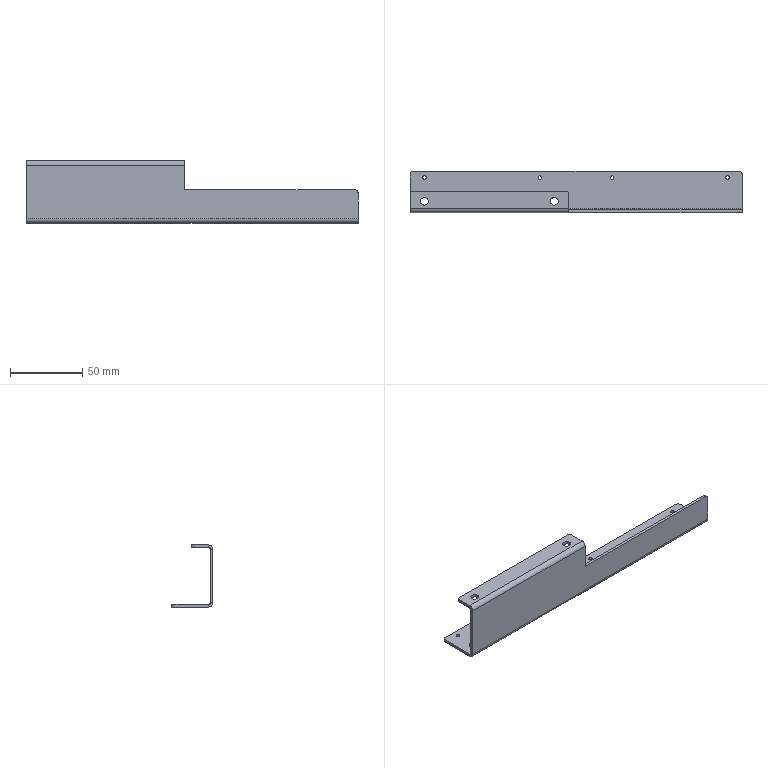Part | SolidWorks | features HoleWzd 2, Cut 1, Fillet 1, FlatPattern 1, SMBaseFlange 1, SheetMetal 1 | 1 solid | 45 faces | box 230 x 29 x 43 mm | volume 29332 mm3 | cylinder 25 | plane 20 | commonest cylinder face diameters 2.5 x8 4 x5 5.5 x4 8 x4 2 x2 6 x2
STEP:
#1=CARTESIAN_POINT('',(11.25,24.5,-19.5));
#2=VERTEX_POINT('',#1);
#3=CARTESIAN_POINT('',(8.75,24.5,-19.5));
#4=VERTEX_POINT('',#3);
#5=CARTESIAN_POINT('',(10.,24.5,-19.5));
#6=DIRECTION('',(0.,0.,-1.));
#7=DIRECTION('',(-1.,0.,0.));
#8=AXIS2_PLACEMENT_3D('',#5,#6,#7);
#9=CIRCLE('',#8,1.25);
#10=EDGE_CURVE('',#2,#4,#9,.T.);
#11=ORIENTED_EDGE('',*,*,#10,.F.);
#12=CARTESIAN_POINT('',(11.25,24.5,-21.5));
#13=VERTEX_POINT('',#12);
#14=CARTESIAN_POINT('',(11.25,24.5,-21.5));
#15=DIRECTION('',(0.,0.,-1.));
#16=VECTOR('',#15,1000.);
#17=LINE('',#14,#16);
#18=EDGE_CURVE('',#2,#13,#17,.T.);
#19=ORIENTED_EDGE('',*,*,#18,.T.);
#20=CARTESIAN_POINT('',(8.75,24.5,-21.5));
#21=VERTEX_POINT('',#20);
#22=CARTESIAN_POINT('',(10.,24.5,-21.5));
#23=DIRECTION('',(0.,0.,-1.));
#24=DIRECTION('',(-1.,0.,0.));
#25=AXIS2_PLACEMENT_3D('',#22,#23,#24);
#26=CIRCLE('',#25,1.25);
#27=EDGE_CURVE('',#13,#21,#26,.T.);
#28=ORIENTED_EDGE('',*,*,#27,.T.);
#29=CARTESIAN_POINT('',(8.75,24.5,-21.5));
#30=DIRECTION('',(0.,0.,-1.));
#31=VECTOR('',#30,1000.);
#32=LINE('',#29,#31);
#33=EDGE_CURVE('',#4,#21,#32,.T.);
#34=ORIENTED_EDGE('',*,*,#33,.F.);
#35=EDGE_LOOP('',(#11,#19,#28,#34));
#36=FACE_OUTER_BOUND('',#35,.T.);
#37=CARTESIAN_POINT('',(10.,24.5,-21.5));
#38=DIRECTION('',(0.,0.,-1.));
#39=DIRECTION('',(-1.,0.,0.));
#40=AXIS2_PLACEMENT_3D('',#37,#38,#39);
#41=CYLINDRICAL_SURFACE('',#40,1.25);
#42=ADVANCED_FACE('',(#36),#41,.F.);
#43=CARTESIAN_POINT('',(91.25,24.5,-19.5));
#44=VERTEX_POINT('',#43);
#45=CARTESIAN_POINT('',(88.75,24.5,-19.5));
#46=VERTEX_POINT('',#45);
#47=CARTESIAN_POINT('',(90.,24.5,-19.5));
#48=DIRECTION('',(0.,0.,-1.));
#49=DIRECTION('',(-1.,0.,0.));
#50=AXIS2_PLACEMENT_3D('',#47,#48,#49);
#51=CIRCLE('',#50,1.25);
#52=EDGE_CURVE('',#44,#46,#51,.T.);
#53=ORIENTED_EDGE('',*,*,#52,.F.);
#54=CARTESIAN_POINT('',(91.25,24.5,-21.5));
#55=VERTEX_POINT('',#54);
#56=CARTESIAN_POINT('',(91.25,24.5,-21.5));
#57=DIRECTION('',(0.,0.,-1.));
#58=VECTOR('',#57,1000.);
#59=LINE('',#56,#58);
#60=EDGE_CURVE('',#44,#55,#59,.T.);
#61=ORIENTED_EDGE('',*,*,#60,.T.);
#62=CARTESIAN_POINT('',(88.75,24.5,-21.5));
#63=VERTEX_POINT('',#62);
#64=CARTESIAN_POINT('',(90.,24.5,-21.5));
#65=DIRECTION('',(0.,0.,-1.));
#66=DIRECTION('',(-1.,0.,0.));
#67=AXIS2_PLACEMENT_3D('',#64,#65,#66);
#68=CIRCLE('',#67,1.25);
#69=EDGE_CURVE('',#55,#63,#68,.T.);
#70=ORIENTED_EDGE('',*,*,#69,.T.);
#71=CARTESIAN_POINT('',(88.75,24.5,-21.5));
#72=DIRECTION('',(0.,0.,-1.));
#73=VECTOR('',#72,1000.);
#74=LINE('',#71,#73);
#75=EDGE_CURVE('',#46,#63,#74,.T.);
#76=ORIENTED_EDGE('',*,*,#75,.F.);
#77=EDGE_LOOP('',(#53,#61,#70,#76));
#78=FACE_OUTER_BOUND('',#77,.T.);
#79=CARTESIAN_POINT('',(90.,24.5,-21.5));
#80=DIRECTION('',(0.,0.,-1.));
#81=DIRECTION('',(-1.,0.,0.));
#82=AXIS2_PLACEMENT_3D('',#79,#80,#81);
#83=CYLINDRICAL_SURFACE('',#82,1.25);
#84=ADVANCED_FACE('',(#78),#83,.F.);
#85=CARTESIAN_POINT('',(141.25,24.5,-19.5));
#86=VERTEX_POINT('',#85);
#87=CARTESIAN_POINT('',(138.75,24.5,-19.5));
#88=VERTEX_POINT('',#87);
#89=CARTESIAN_POINT('',(140.,24.5,-19.5));
#90=DIRECTION('',(0.,0.,-1.));
#91=DIRECTION('',(-1.,0.,0.));
#92=AXIS2_PLACEMENT_3D('',#89,#90,#91);
#93=CIRCLE('',#92,1.25);
#94=EDGE_CURVE('',#86,#88,#93,.T.);
#95=ORIENTED_EDGE('',*,*,#94,.F.);
#96=CARTESIAN_POINT('',(141.25,24.5,-21.5));
#97=VERTEX_POINT('',#96);
#98=CARTESIAN_POINT('',(141.25,24.5,-21.5));
#99=DIRECTION('',(0.,0.,-1.));
#100=VECTOR('',#99,1000.);
#101=LINE('',#98,#100);
#102=EDGE_CURVE('',#86,#97,#101,.T.);
#103=ORIENTED_EDGE('',*,*,#102,.T.);
#104=CARTESIAN_POINT('',(138.75,24.5,-21.5));
#105=VERTEX_POINT('',#104);
#106=CARTESIAN_POINT('',(140.,24.5,-21.5));
#107=DIRECTION('',(0.,0.,-1.));
#108=DIRECTION('',(-1.,0.,0.));
#109=AXIS2_PLACEMENT_3D('',#106,#107,#108);
#110=CIRCLE('',#109,1.25);
#111=EDGE_CURVE('',#97,#105,#110,.T.);
#112=ORIENTED_EDGE('',*,*,#111,.T.);
#113=CARTESIAN_POINT('',(138.75,24.5,-21.5));
#114=DIRECTION('',(0.,0.,-1.));
#115=VECTOR('',#114,1000.);
#116=LINE('',#113,#115);
#117=EDGE_CURVE('',#88,#105,#116,.T.);
#118=ORIENTED_EDGE('',*,*,#117,.F.);
#119=EDGE_LOOP('',(#95,#103,#112,#118));
#120=FACE_OUTER_BOUND('',#119,.T.);
#121=CARTESIAN_POINT('',(140.,24.5,-21.5));
#122=DIRECTION('',(0.,0.,-1.));
#123=DIRECTION('',(-1.,0.,0.));
#124=AXIS2_PLACEMENT_3D('',#121,#122,#123);
#125=CYLINDRICAL_SURFACE('',#124,1.25);
#126=ADVANCED_FACE('',(#120),#125,.F.);
#127=CARTESIAN_POINT('',(221.25,24.5,-19.5));
#128=VERTEX_POINT('',#127);
#129=CARTESIAN_POINT('',(218.75,24.5,-19.5));
#130=VERTEX_POINT('',#129);
#131=CARTESIAN_POINT('',(220.,24.5,-19.5));
#132=DIRECTION('',(0.,0.,-1.));
#133=DIRECTION('',(-1.,0.,0.));
#134=AXIS2_PLACEMENT_3D('',#131,#132,#133);
#135=CIRCLE('',#134,1.25);
#136=EDGE_CURVE('',#128,#130,#135,.T.);
#137=ORIENTED_EDGE('',*,*,#136,.F.);
#138=CARTESIAN_POINT('',(221.25,24.5,-21.5));
#139=VERTEX_POINT('',#138);
#140=CARTESIAN_POINT('',(221.25,24.5,-21.5));
#141=DIRECTION('',(0.,0.,-1.));
#142=VECTOR('',#141,1000.);
#143=LINE('',#140,#142);
#144=EDGE_CURVE('',#128,#139,#143,.T.);
#145=ORIENTED_EDGE('',*,*,#144,.T.);
#146=CARTESIAN_POINT('',(218.75,24.5,-21.5));
#147=VERTEX_POINT('',#146);
#148=CARTESIAN_POINT('',(220.,24.5,-21.5));
#149=DIRECTION('',(0.,0.,-1.));
#150=DIRECTION('',(-1.,0.,0.));
#151=AXIS2_PLACEMENT_3D('',#148,#149,#150);
#152=CIRCLE('',#151,1.25);
#153=EDGE_CURVE('',#139,#147,#152,.T.);
#154=ORIENTED_EDGE('',*,*,#153,.T.);
#155=CARTESIAN_POINT('',(218.75,24.5,-21.5));
#156=DIRECTION('',(0.,0.,-1.));
#157=VECTOR('',#156,1000.);
#158=LINE('',#155,#157);
#159=EDGE_CURVE('',#130,#147,#158,.T.);
#160=ORIENTED_EDGE('',*,*,#159,.F.);
#161=EDGE_LOOP('',(#137,#145,#154,#160));
#162=FACE_OUTER_BOUND('',#161,.T.);
#163=CARTESIAN_POINT('',(220.,24.5,-21.5));
#164=DIRECTION('',(0.,0.,-1.));
#165=DIRECTION('',(-1.,0.,0.));
#166=AXIS2_PLACEMENT_3D('',#163,#164,#165);
#167=CYLINDRICAL_SURFACE('',#166,1.25);
#168=ADVANCED_FACE('',(#162),#167,.F.);
#169=CARTESIAN_POINT('',(12.75,8.,21.5));
#170=VERTEX_POINT('',#169);
#171=CARTESIAN_POINT('',(7.25,8.,21.5));
#172=VERTEX_POINT('',#171);
#173=CARTESIAN_POINT('',(10.,8.,21.5));
#174=DIRECTION('',(0.,0.,-1.));
#175=DIRECTION('',(-1.,0.,0.));
#176=AXIS2_PLACEMENT_3D('',#173,#174,#175);
#177=CIRCLE('',#176,2.75);
#178=EDGE_CURVE('',#170,#172,#177,.T.);
#179=ORIENTED_EDGE('',*,*,#178,.F.);
#180=CARTESIAN_POINT('',(12.75,8.,19.5));
#181=VERTEX_POINT('',#180);
#182=CARTESIAN_POINT('',(12.75,8.,-21.5));
#183=DIRECTION('',(0.,0.,-1.));
#184=VECTOR('',#183,1000.);
#185=LINE('',#182,#184);
#186=EDGE_CURVE('',#170,#181,#185,.T.);
#187=ORIENTED_EDGE('',*,*,#186,.T.);
#188=CARTESIAN_POINT('',(7.25,8.,19.5));
#189=VERTEX_POINT('',#188);
#190=CARTESIAN_POINT('',(10.,8.,19.5));
#191=DIRECTION('',(0.,0.,1.));
#192=DIRECTION('',(1.,0.,0.));
#193=AXIS2_PLACEMENT_3D('',#190,#191,#192);
#194=CIRCLE('',#193,2.75);
#195=EDGE_CURVE('',#189,#181,#194,.T.);
#196=ORIENTED_EDGE('',*,*,#195,.F.);
#197=CARTESIAN_POINT('',(7.25,8.,-21.5));
#198=DIRECTION('',(0.,0.,-1.));
#199=VECTOR('',#198,1000.);
#200=LINE('',#197,#199);
#201=EDGE_CURVE('',#172,#189,#200,.T.);
#202=ORIENTED_EDGE('',*,*,#201,.F.);
#203=EDGE_LOOP('',(#179,#187,#196,#202));
#204=FACE_OUTER_BOUND('',#203,.T.);
#205=CARTESIAN_POINT('',(10.,8.,-21.5));
#206=DIRECTION('',(0.,0.,-1.));
#207=DIRECTION('',(-1.,0.,0.));
#208=AXIS2_PLACEMENT_3D('',#205,#206,#207);
#209=CYLINDRICAL_SURFACE('',#208,2.75);
#210=ADVANCED_FACE('',(#204),#209,.F.);
#211=CARTESIAN_POINT('',(14.,8.,-19.5));
#212=VERTEX_POINT('',#211);
#213=CARTESIAN_POINT('',(6.,8.,-19.5));
#214=VERTEX_POINT('',#213);
#215=CARTESIAN_POINT('',(10.,8.,-19.5));
#216=DIRECTION('',(0.,0.,-1.));
#217=DIRECTION('',(-1.,0.,0.));
#218=AXIS2_PLACEMENT_3D('',#215,#216,#217);
#219=CIRCLE('',#218,4.);
#220=EDGE_CURVE('',#212,#214,#219,.T.);
#221=ORIENTED_EDGE('',*,*,#220,.F.);
#222=CARTESIAN_POINT('',(14.,8.,-21.5));
#223=VERTEX_POINT('',#222);
#224=CARTESIAN_POINT('',(14.,8.,-21.5));
#225=DIRECTION('',(0.,0.,-1.));
#226=VECTOR('',#225,1000.);
#227=LINE('',#224,#226);
#228=EDGE_CURVE('',#212,#223,#227,.T.);
#229=ORIENTED_EDGE('',*,*,#228,.T.);
#230=CARTESIAN_POINT('',(6.,8.,-21.5));
#231=VERTEX_POINT('',#230);
#232=CARTESIAN_POINT('',(10.,8.,-21.5));
#233=DIRECTION('',(0.,0.,-1.));
#234=DIRECTION('',(-1.,0.,0.));
#235=AXIS2_PLACEMENT_3D('',#232,#233,#234);
#236=CIRCLE('',#235,4.);
#237=EDGE_CURVE('',#223,#231,#236,.T.);
#238=ORIENTED_EDGE('',*,*,#237,.T.);
#239=CARTESIAN_POINT('',(6.,8.,-21.5));
#240=DIRECTION('',(0.,0.,-1.));
#241=VECTOR('',#240,1000.);
#242=LINE('',#239,#241);
#243=EDGE_CURVE('',#214,#231,#242,.T.);
#244=ORIENTED_EDGE('',*,*,#243,.F.);
#245=EDGE_LOOP('',(#221,#229,#238,#244));
#246=FACE_OUTER_BOUND('',#245,.T.);
#247=CARTESIAN_POINT('',(10.,8.,-21.5));
#248=DIRECTION('',(0.,0.,-1.));
#249=DIRECTION('',(-1.,0.,0.));
#250=AXIS2_PLACEMENT_3D('',#247,#248,#249);
#251=CYLINDRICAL_SURFACE('',#250,4.);
#252=ADVANCED_FACE('',(#246),#251,.F.);
#253=CARTESIAN_POINT('',(102.75,8.,21.5));
#254=VERTEX_POINT('',#253);
#255=CARTESIAN_POINT('',(97.25,8.,21.5));
#256=VERTEX_POINT('',#255);
#257=CARTESIAN_POINT('',(100.,8.,21.5));
#258=DIRECTION('',(0.,0.,-1.));
#259=DIRECTION('',(-1.,0.,0.));
#260=AXIS2_PLACEMENT_3D('',#257,#258,#259);
#261=CIRCLE('',#260,2.75);
#262=EDGE_CURVE('',#254,#256,#261,.T.);
#263=ORIENTED_EDGE('',*,*,#262,.F.);
#264=CARTESIAN_POINT('',(102.75,8.,19.5));
#265=VERTEX_POINT('',#264);
#266=CARTESIAN_POINT('',(102.75,8.,-21.5));
#267=DIRECTION('',(0.,0.,-1.));
#268=VECTOR('',#267,1000.);
#269=LINE('',#266,#268);
#270=EDGE_CURVE('',#254,#265,#269,.T.);
#271=ORIENTED_EDGE('',*,*,#270,.T.);
#272=CARTESIAN_POINT('',(97.25,8.,19.5));
#273=VERTEX_POINT('',#272);
#274=CARTESIAN_POINT('',(100.,8.,19.5));
#275=DIRECTION('',(0.,0.,1.));
#276=DIRECTION('',(1.,0.,0.));
#277=AXIS2_PLACEMENT_3D('',#274,#275,#276);
#278=CIRCLE('',#277,2.75);
#279=EDGE_CURVE('',#273,#265,#278,.T.);
#280=ORIENTED_EDGE('',*,*,#279,.F.);
#281=CARTESIAN_POINT('',(97.25,8.,-21.5));
#282=DIRECTION('',(0.,0.,-1.));
#283=VECTOR('',#282,1000.);
#284=LINE('',#281,#283);
#285=EDGE_CURVE('',#256,#273,#284,.T.);
#286=ORIENTED_EDGE('',*,*,#285,.F.);
#287=EDGE_LOOP('',(#263,#271,#280,#286));
#288=FACE_OUTER_BOUND('',#287,.T.);
#289=CARTESIAN_POINT('',(100.,8.,-21.5));
#290=DIRECTION('',(0.,0.,-1.));
#291=DIRECTION('',(-1.,0.,0.));
#292=AXIS2_PLACEMENT_3D('',#289,#290,#291);
#293=CYLINDRICAL_SURFACE('',#292,2.75);
#294=ADVANCED_FACE('',(#288),#293,.F.);
#295=CARTESIAN_POINT('',(104.,8.,-19.5));
#296=VERTEX_POINT('',#295);
#297=CARTESIAN_POINT('',(96.,8.,-19.5));
#298=VERTEX_POINT('',#297);
#299=CARTESIAN_POINT('',(100.,8.,-19.5));
#300=DIRECTION('',(0.,0.,-1.));
#301=DIRECTION('',(-1.,0.,0.));
#302=AXIS2_PLACEMENT_3D('',#299,#300,#301);
#303=CIRCLE('',#302,4.);
#304=EDGE_CURVE('',#296,#298,#303,.T.);
#305=ORIENTED_EDGE('',*,*,#304,.F.);
#306=CARTESIAN_POINT('',(104.,8.,-21.5));
#307=VERTEX_POINT('',#306);
#308=CARTESIAN_POINT('',(104.,8.,-21.5));
#309=DIRECTION('',(0.,0.,-1.));
#310=VECTOR('',#309,1000.);
#311=LINE('',#308,#310);
#312=EDGE_CURVE('',#296,#307,#311,.T.);
#313=ORIENTED_EDGE('',*,*,#312,.T.);
#314=CARTESIAN_POINT('',(96.,8.,-21.5));
#315=VERTEX_POINT('',#314);
#316=CARTESIAN_POINT('',(100.,8.,-21.5));
#317=DIRECTION('',(0.,0.,-1.));
#318=DIRECTION('',(-1.,0.,0.));
#319=AXIS2_PLACEMENT_3D('',#316,#317,#318);
#320=CIRCLE('',#319,4.);
#321=EDGE_CURVE('',#307,#315,#320,.T.);
#322=ORIENTED_EDGE('',*,*,#321,.T.);
#323=CARTESIAN_POINT('',(96.,8.,-21.5));
#324=DIRECTION('',(0.,0.,-1.));
#325=VECTOR('',#324,1000.);
#326=LINE('',#323,#325);
#327=EDGE_CURVE('',#298,#315,#326,.T.);
#328=ORIENTED_EDGE('',*,*,#327,.F.);
#329=EDGE_LOOP('',(#305,#313,#322,#328));
#330=FACE_OUTER_BOUND('',#329,.T.);
#331=CARTESIAN_POINT('',(100.,8.,-21.5));
#332=DIRECTION('',(0.,0.,-1.));
#333=DIRECTION('',(-1.,0.,0.));
#334=AXIS2_PLACEMENT_3D('',#331,#332,#333);
#335=CYLINDRICAL_SURFACE('',#334,4.);
#336=ADVANCED_FACE('',(#330),#335,.F.);
#337=CARTESIAN_POINT('',(110.,2.,18.5));
#338=VERTEX_POINT('',#337);
#339=CARTESIAN_POINT('',(110.,2.,1.5));
#340=VERTEX_POINT('',#339);
#341=CARTESIAN_POINT('',(110.,2.,21.5));
#342=DIRECTION('',(0.,0.,-1.));
#343=VECTOR('',#342,1000.);
#344=LINE('',#341,#343);
#345=EDGE_CURVE('',#338,#340,#344,.T.);
#346=ORIENTED_EDGE('',*,*,#345,.F.);
#347=CARTESIAN_POINT('',(110.,0.,18.5));
#348=VERTEX_POINT('',#347);
#349=CARTESIAN_POINT('',(110.,2.,18.5));
#350=DIRECTION('',(0.,-1.,0.));
#351=VECTOR('',#350,1000.);
#352=LINE('',#349,#351);
#353=EDGE_CURVE('',#338,#348,#352,.T.);
#354=ORIENTED_EDGE('',*,*,#353,.T.);
#355=CARTESIAN_POINT('',(110.,0.,1.5));
#356=VERTEX_POINT('',#355);
#357=CARTESIAN_POINT('',(110.,0.,21.5));
#358=DIRECTION('',(0.,0.,-1.));
#359=VECTOR('',#358,1000.);
#360=LINE('',#357,#359);
#361=EDGE_CURVE('',#348,#356,#360,.T.);
#362=ORIENTED_EDGE('',*,*,#361,.T.);
#363=CARTESIAN_POINT('',(110.,29.,1.5));
#364=DIRECTION('',(0.,-1.,0.));
#365=VECTOR('',#364,1000.);
#366=LINE('',#363,#365);
#367=EDGE_CURVE('',#340,#356,#366,.T.);
#368=ORIENTED_EDGE('',*,*,#367,.F.);
#369=EDGE_LOOP('',(#346,#354,#362,#368));
#370=FACE_OUTER_BOUND('',#369,.T.);
#371=CARTESIAN_POINT('',(110.,29.,21.5));
#372=DIRECTION('',(-1.,0.,0.));
#373=DIRECTION('',(0.,0.,1.));
#374=AXIS2_PLACEMENT_3D('',#371,#372,#373);
#375=PLANE('',#374);
#376=ADVANCED_FACE('',(#370),#375,.F.);
#377=CARTESIAN_POINT('',(110.,13.,19.5));
#378=VERTEX_POINT('',#377);
#379=CARTESIAN_POINT('',(110.,3.,19.5));
#380=VERTEX_POINT('',#379);
#381=CARTESIAN_POINT('',(110.,0.,19.5));
#382=DIRECTION('',(0.,-1.,0.));
#383=VECTOR('',#382,1000.);
#384=LINE('',#381,#383);
#385=EDGE_CURVE('',#378,#380,#384,.T.);
#386=ORIENTED_EDGE('',*,*,#385,.F.);
#387=CARTESIAN_POINT('',(110.,13.,21.5));
#388=VERTEX_POINT('',#387);
#389=CARTESIAN_POINT('',(110.,13.,21.5));
#390=DIRECTION('',(0.,0.,1.));
#391=VECTOR('',#390,1000.);
#392=LINE('',#389,#391);
#393=EDGE_CURVE('',#378,#388,#392,.T.);
#394=ORIENTED_EDGE('',*,*,#393,.T.);
#395=CARTESIAN_POINT('',(110.,3.,21.5));
#396=VERTEX_POINT('',#395);
#397=CARTESIAN_POINT('',(110.,29.,21.5));
#398=DIRECTION('',(0.,-1.,0.));
#399=VECTOR('',#398,1000.);
#400=LINE('',#397,#399);
#401=EDGE_CURVE('',#388,#396,#400,.T.);
#402=ORIENTED_EDGE('',*,*,#401,.T.);
#403=CARTESIAN_POINT('',(110.,3.,21.5));
#404=DIRECTION('',(0.,0.,-1.));
#405=VECTOR('',#404,1000.);
#406=LINE('',#403,#405);
#407=EDGE_CURVE('',#396,#380,#406,.T.);
#408=ORIENTED_EDGE('',*,*,#407,.T.);
#409=EDGE_LOOP('',(#386,#394,#402,#408));
#410=FACE_OUTER_BOUND('',#409,.T.);
#411=CARTESIAN_POINT('',(110.,29.,21.5));
#412=DIRECTION('',(-1.,0.,0.));
#413=DIRECTION('',(0.,0.,1.));
#414=AXIS2_PLACEMENT_3D('',#411,#412,#413);
#415=PLANE('',#414);
#416=ADVANCED_FACE('',(#410),#415,.F.);
#417=CARTESIAN_POINT('',(230.,0.,-18.5));
#418=VERTEX_POINT('',#417);
#419=CARTESIAN_POINT('',(230.,2.,-18.5));
#420=VERTEX_POINT('',#419);
#421=CARTESIAN_POINT('',(230.,0.,-18.5));
#422=DIRECTION('',(0.,1.,0.));
#423=VECTOR('',#422,1000.);
#424=LINE('',#421,#423);
#425=EDGE_CURVE('',#418,#420,#424,.T.);
#426=ORIENTED_EDGE('',*,*,#425,.F.);
#427=CARTESIAN_POINT('',(230.,3.,-21.5));
#428=VERTEX_POINT('',#427);
#429=CARTESIAN_POINT('',(230.,3.,-18.5));
#430=DIRECTION('',(-1.,0.,0.));
#431=DIRECTION('',(0.,0.,-1.));
#432=AXIS2_PLACEMENT_3D('',#429,#430,#431);
#433=CIRCLE('',#432,3.);
#434=EDGE_CURVE('',#428,#418,#433,.T.);
#435=ORIENTED_EDGE('',*,*,#434,.F.);
#436=CARTESIAN_POINT('',(230.,3.,-19.5));
#437=VERTEX_POINT('',#436);
#438=CARTESIAN_POINT('',(230.,3.,-19.5));
#439=DIRECTION('',(0.,0.,-1.));
#440=VECTOR('',#439,1000.);
#441=LINE('',#438,#440);
#442=EDGE_CURVE('',#437,#428,#441,.T.);
#443=ORIENTED_EDGE('',*,*,#442,.F.);
#444=CARTESIAN_POINT('',(230.,3.,-18.5));
#445=DIRECTION('',(-1.,0.,0.));
#446=DIRECTION('',(0.,0.,-1.));
#447=AXIS2_PLACEMENT_3D('',#444,#445,#446);
#448=CIRCLE('',#447,1.);
#449=EDGE_CURVE('',#437,#420,#448,.T.);
#450=ORIENTED_EDGE('',*,*,#449,.T.);
#451=EDGE_LOOP('',(#426,#435,#443,#450));
#452=FACE_OUTER_BOUND('',#451,.T.);
#453=CARTESIAN_POINT('',(230.,0.,-18.5));
#454=DIRECTION('',(1.,0.,0.));
#455=DIRECTION('',(0.,0.,-1.));
#456=AXIS2_PLACEMENT_3D('',#453,#454,#455);
#457=PLANE('',#456);
#458=ADVANCED_FACE('',(#452),#457,.T.);
#459=CARTESIAN_POINT('',(230.,2.,-0.5));
#460=VERTEX_POINT('',#459);
#461=CARTESIAN_POINT('',(230.,2.,21.5));
#462=DIRECTION('',(0.,0.,1.));
#463=VECTOR('',#462,1000.);
#464=LINE('',#461,#463);
#465=EDGE_CURVE('',#420,#460,#464,.T.);
#466=ORIENTED_EDGE('',*,*,#465,.T.);
#467=CARTESIAN_POINT('',(230.,0.,-0.5));
#468=VERTEX_POINT('',#467);
#469=CARTESIAN_POINT('',(230.,0.,-0.5));
#470=DIRECTION('',(0.,-1.,0.));
#471=VECTOR('',#470,1000.);
#472=LINE('',#469,#471);
#473=EDGE_CURVE('',#460,#468,#472,.T.);
#474=ORIENTED_EDGE('',*,*,#473,.T.);
#475=CARTESIAN_POINT('',(230.,0.,21.5));
#476=DIRECTION('',(0.,0.,1.));
#477=VECTOR('',#476,1000.);
#478=LINE('',#475,#477);
#479=EDGE_CURVE('',#418,#468,#478,.T.);
#480=ORIENTED_EDGE('',*,*,#479,.F.);
#481=ORIENTED_EDGE('',*,*,#425,.T.);
#482=EDGE_LOOP('',(#466,#474,#480,#481));
#483=FACE_OUTER_BOUND('',#482,.T.);
#484=CARTESIAN_POINT('',(230.,3.,-19.5));
#485=DIRECTION('',(1.,0.,0.));
#486=DIRECTION('',(0.,0.,-1.));
#487=AXIS2_PLACEMENT_3D('',#484,#485,#486);
#488=PLANE('',#487);
#489=ADVANCED_FACE('',(#483),#488,.T.);
#490=CARTESIAN_POINT('',(0.,3.,-21.5));
#491=VERTEX_POINT('',#490);
#492=CARTESIAN_POINT('',(0.,3.,-19.5));
#493=VERTEX_POINT('',#492);
#494=CARTESIAN_POINT('',(0.,3.,-21.5));
#495=DIRECTION('',(0.,0.,1.));
#496=VECTOR('',#495,1000.);
#497=LINE('',#494,#496);
#498=EDGE_CURVE('',#491,#493,#497,.T.);
#499=ORIENTED_EDGE('',*,*,#498,.F.);
#500=CARTESIAN_POINT('',(0.,0.,-18.5));
#501=VERTEX_POINT('',#500);
#502=CARTESIAN_POINT('',(0.,3.,-18.5));
#503=DIRECTION('',(-1.,0.,0.));
#504=DIRECTION('',(0.,0.,-1.));
#505=AXIS2_PLACEMENT_3D('',#502,#503,#504);
#506=CIRCLE('',#505,3.);
#507=EDGE_CURVE('',#491,#501,#506,.T.);
#508=ORIENTED_EDGE('',*,*,#507,.T.);
#509=CARTESIAN_POINT('',(0.,2.,-18.5));
#510=VERTEX_POINT('',#509);
#511=CARTESIAN_POINT('',(0.,2.,-18.5));
#512=DIRECTION('',(0.,-1.,0.));
#513=VECTOR('',#512,1000.);
#514=LINE('',#511,#513);
#515=EDGE_CURVE('',#510,#501,#514,.T.);
#516=ORIENTED_EDGE('',*,*,#515,.F.);
#517=CARTESIAN_POINT('',(0.,3.,-18.5));
#518=DIRECTION('',(-1.,0.,0.));
#519=DIRECTION('',(0.,0.,-1.));
#520=AXIS2_PLACEMENT_3D('',#517,#518,#519);
#521=CIRCLE('',#520,1.);
#522=EDGE_CURVE('',#493,#510,#521,.T.);
#523=ORIENTED_EDGE('',*,*,#522,.F.);
#524=EDGE_LOOP('',(#499,#508,#516,#523));
#525=FACE_OUTER_BOUND('',#524,.T.);
#526=CARTESIAN_POINT('',(0.,3.,-21.5));
#527=DIRECTION('',(-1.,0.,0.));
#528=DIRECTION('',(0.,0.,1.));
#529=AXIS2_PLACEMENT_3D('',#526,#527,#528);
#530=PLANE('',#529);
#531=ADVANCED_FACE('',(#525),#530,.T.);
#532=CARTESIAN_POINT('',(0.,27.,-19.5));
#533=VERTEX_POINT('',#532);
#534=CARTESIAN_POINT('',(0.,0.,-19.5));
#535=DIRECTION('',(0.,-1.,0.));
#536=VECTOR('',#535,1000.);
#537=LINE('',#534,#536);
#538=EDGE_CURVE('',#533,#493,#537,.T.);
#539=ORIENTED_EDGE('',*,*,#538,.F.);
#540=CARTESIAN_POINT('',(0.,27.,-21.5));
#541=VERTEX_POINT('',#540);
#542=CARTESIAN_POINT('',(0.,27.,-18.5));
#543=DIRECTION('',(0.,0.,-1.));
#544=VECTOR('',#543,1000.);
#545=LINE('',#542,#544);
#546=EDGE_CURVE('',#533,#541,#545,.T.);
#547=ORIENTED_EDGE('',*,*,#546,.T.);
#548=CARTESIAN_POINT('',(0.,0.,-21.5));
#549=DIRECTION('',(0.,-1.,0.));
#550=VECTOR('',#549,1000.);
#551=LINE('',#548,#550);
#552=EDGE_CURVE('',#541,#491,#551,.T.);
#553=ORIENTED_EDGE('',*,*,#552,.T.);
#554=ORIENTED_EDGE('',*,*,#498,.T.);
#555=EDGE_LOOP('',(#539,#547,#553,#554));
#556=FACE_OUTER_BOUND('',#555,.T.);
#557=CARTESIAN_POINT('',(0.,2.,-18.5));
#558=DIRECTION('',(-1.,0.,0.));
#559=DIRECTION('',(0.,0.,1.));
#560=AXIS2_PLACEMENT_3D('',#557,#558,#559);
#561=PLANE('',#560);
#562=ADVANCED_FACE('',(#556),#561,.T.);
#563=CARTESIAN_POINT('',(0.,0.,18.5));
#564=VERTEX_POINT('',#563);
#565=CARTESIAN_POINT('',(0.,2.,18.5));
#566=VERTEX_POINT('',#565);
#567=CARTESIAN_POINT('',(0.,0.,18.5));
#568=DIRECTION('',(0.,1.,0.));
#569=VECTOR('',#568,1000.);
#570=LINE('',#567,#569);
#571=EDGE_CURVE('',#564,#566,#570,.T.);
#572=ORIENTED_EDGE('',*,*,#571,.F.);
#573=CARTESIAN_POINT('',(0.,3.,21.5));
#574=VERTEX_POINT('',#573);
#575=CARTESIAN_POINT('',(0.,3.,18.5));
#576=DIRECTION('',(-1.,0.,0.));
#577=DIRECTION('',(0.,0.,-1.));
#578=AXIS2_PLACEMENT_3D('',#575,#576,#577);
#579=CIRCLE('',#578,3.);
#580=EDGE_CURVE('',#564,#574,#579,.T.);
#581=ORIENTED_EDGE('',*,*,#580,.T.);
#582=CARTESIAN_POINT('',(0.,3.,19.5));
#583=VERTEX_POINT('',#582);
#584=CARTESIAN_POINT('',(0.,3.,19.5));
#585=DIRECTION('',(0.,0.,1.));
#586=VECTOR('',#585,1000.);
#587=LINE('',#584,#586);
#588=EDGE_CURVE('',#583,#574,#587,.T.);
#589=ORIENTED_EDGE('',*,*,#588,.F.);
#590=CARTESIAN_POINT('',(0.,3.,18.5));
#591=DIRECTION('',(-1.,0.,0.));
#592=DIRECTION('',(0.,0.,-1.));
#593=AXIS2_PLACEMENT_3D('',#590,#591,#592);
#594=CIRCLE('',#593,1.);
#595=EDGE_CURVE('',#566,#583,#594,.T.);
#596=ORIENTED_EDGE('',*,*,#595,.F.);
#597=EDGE_LOOP('',(#572,#581,#589,#596));
#598=FACE_OUTER_BOUND('',#597,.T.);
#599=CARTESIAN_POINT('',(0.,0.,18.5));
#600=DIRECTION('',(-1.,0.,0.));
#601=DIRECTION('',(0.,0.,1.));
#602=AXIS2_PLACEMENT_3D('',#599,#600,#601);
#603=PLANE('',#602);
#604=ADVANCED_FACE('',(#598),#603,.T.);
#605=CARTESIAN_POINT('',(0.,0.,21.5));
#606=DIRECTION('',(0.,0.,1.));
#607=VECTOR('',#606,1000.);
#608=LINE('',#605,#607);
#609=EDGE_CURVE('',#501,#564,#608,.T.);
#610=ORIENTED_EDGE('',*,*,#609,.T.);
#611=ORIENTED_EDGE('',*,*,#571,.T.);
#612=CARTESIAN_POINT('',(0.,2.,21.5));
#613=DIRECTION('',(0.,0.,1.));
#614=VECTOR('',#613,1000.);
#615=LINE('',#612,#614);
#616=EDGE_CURVE('',#510,#566,#615,.T.);
#617=ORIENTED_EDGE('',*,*,#616,.F.);
#618=ORIENTED_EDGE('',*,*,#515,.T.);
#619=EDGE_LOOP('',(#610,#611,#617,#618));
#620=FACE_OUTER_BOUND('',#619,.T.);
#621=CARTESIAN_POINT('',(0.,3.,19.5));
#622=DIRECTION('',(-1.,0.,0.));
#623=DIRECTION('',(0.,0.,1.));
#624=AXIS2_PLACEMENT_3D('',#621,#622,#623);
#625=PLANE('',#624);
#626=ADVANCED_FACE('',(#620),#625,.T.);
#627=ORIENTED_EDGE('',*,*,#195,.T.);
#628=CARTESIAN_POINT('',(10.,8.,19.5));
#629=DIRECTION('',(0.,0.,1.));
#630=DIRECTION('',(1.,0.,0.));
#631=AXIS2_PLACEMENT_3D('',#628,#629,#630);
#632=CIRCLE('',#631,2.75);
#633=EDGE_CURVE('',#181,#189,#632,.T.);
#634=ORIENTED_EDGE('',*,*,#633,.T.);
#635=EDGE_LOOP('',(#627,#634));
#636=FACE_BOUND('',#635,.T.);
#637=ORIENTED_EDGE('',*,*,#279,.T.);
#638=CARTESIAN_POINT('',(100.,8.,19.5));
#639=DIRECTION('',(0.,0.,1.));
#640=DIRECTION('',(1.,0.,0.));
#641=AXIS2_PLACEMENT_3D('',#638,#639,#640);
#642=CIRCLE('',#641,2.75);
#643=EDGE_CURVE('',#265,#273,#642,.T.);
#644=ORIENTED_EDGE('',*,*,#643,.T.);
#645=EDGE_LOOP('',(#637,#644));
#646=FACE_BOUND('',#645,.T.);
#647=CARTESIAN_POINT('',(108.,15.,19.5));
#648=VERTEX_POINT('',#647);
#649=CARTESIAN_POINT('',(2.,15.,19.5));
#650=VERTEX_POINT('',#649);
#651=CARTESIAN_POINT('',(230.,15.,19.5));
#652=DIRECTION('',(-1.,0.,0.));
#653=VECTOR('',#652,1000.);
#654=LINE('',#651,#653);
#655=EDGE_CURVE('',#648,#650,#654,.T.);
#656=ORIENTED_EDGE('',*,*,#655,.F.);
#657=CARTESIAN_POINT('',(108.,13.,19.5));
#658=DIRECTION('',(0.,0.,-1.));
#659=DIRECTION('',(1.,0.,0.));
#660=AXIS2_PLACEMENT_3D('',#657,#658,#659);
#661=CIRCLE('',#660,2.);
#662=EDGE_CURVE('',#648,#378,#661,.T.);
#663=ORIENTED_EDGE('',*,*,#662,.T.);
#664=ORIENTED_EDGE('',*,*,#385,.T.);
#665=CARTESIAN_POINT('',(230.,3.,19.5));
#666=DIRECTION('',(-1.,0.,0.));
#667=VECTOR('',#666,1000.);
#668=LINE('',#665,#667);
#669=EDGE_CURVE('',#380,#583,#668,.T.);
#670=ORIENTED_EDGE('',*,*,#669,.T.);
#671=CARTESIAN_POINT('',(0.,13.,19.5));
#672=VERTEX_POINT('',#671);
#673=CARTESIAN_POINT('',(0.,0.,19.5));
#674=DIRECTION('',(0.,1.,0.));
#675=VECTOR('',#674,1000.);
#676=LINE('',#673,#675);
#677=EDGE_CURVE('',#583,#672,#676,.T.);
#678=ORIENTED_EDGE('',*,*,#677,.T.);
#679=CARTESIAN_POINT('',(2.,13.,19.5));
#680=DIRECTION('',(0.,0.,-1.));
#681=DIRECTION('',(1.,0.,0.));
#682=AXIS2_PLACEMENT_3D('',#679,#680,#681);
#683=CIRCLE('',#682,2.);
#684=EDGE_CURVE('',#672,#650,#683,.T.);
#685=ORIENTED_EDGE('',*,*,#684,.T.);
#686=EDGE_LOOP('',(#656,#663,#664,#670,#678,#685));
#687=FACE_OUTER_BOUND('',#686,.T.);
#688=CARTESIAN_POINT('',(230.,0.,19.5));
#689=DIRECTION('',(0.,0.,1.));
#690=DIRECTION('',(1.,0.,0.));
#691=AXIS2_PLACEMENT_3D('',#688,#689,#690);
#692=PLANE('',#691);
#693=ADVANCED_FACE('',(#636,#646,#687),#692,.F.);
#694=CARTESIAN_POINT('',(108.,15.,21.5));
#695=VERTEX_POINT('',#694);
#696=CARTESIAN_POINT('',(2.,15.,21.5));
#697=VERTEX_POINT('',#696);
#698=CARTESIAN_POINT('',(230.,15.,21.5));
#699=DIRECTION('',(-1.,0.,0.));
#700=VECTOR('',#699,1000.);
#701=LINE('',#698,#700);
#702=EDGE_CURVE('',#695,#697,#701,.T.);
#703=ORIENTED_EDGE('',*,*,#702,.F.);
#704=CARTESIAN_POINT('',(108.,15.,19.5));
#705=DIRECTION('',(0.,0.,-1.));
#706=VECTOR('',#705,1000.);
#707=LINE('',#704,#706);
#708=EDGE_CURVE('',#695,#648,#707,.T.);
#709=ORIENTED_EDGE('',*,*,#708,.T.);
#710=ORIENTED_EDGE('',*,*,#655,.T.);
#711=CARTESIAN_POINT('',(2.,15.,21.5));
#712=DIRECTION('',(0.,0.,1.));
#713=VECTOR('',#712,1000.);
#714=LINE('',#711,#713);
#715=EDGE_CURVE('',#650,#697,#714,.T.);
#716=ORIENTED_EDGE('',*,*,#715,.T.);
#717=EDGE_LOOP('',(#703,#709,#710,#716));
#718=FACE_OUTER_BOUND('',#717,.T.);
#719=CARTESIAN_POINT('',(230.,15.,21.5));
#720=DIRECTION('',(0.,1.,0.));
#721=DIRECTION('',(0.,0.,1.));
#722=AXIS2_PLACEMENT_3D('',#719,#720,#721);
#723=PLANE('',#722);
#724=ADVANCED_FACE('',(#718),#723,.T.);
#725=CARTESIAN_POINT('',(10.,8.,21.5));
#726=DIRECTION('',(0.,0.,-1.));
#727=DIRECTION('',(-1.,0.,0.));
#728=AXIS2_PLACEMENT_3D('',#725,#726,#727);
#729=CIRCLE('',#728,2.75);
#730=EDGE_CURVE('',#172,#170,#729,.T.);
#731=ORIENTED_EDGE('',*,*,#730,.T.);
#732=ORIENTED_EDGE('',*,*,#178,.T.);
#733=EDGE_LOOP('',(#731,#732));
#734=FACE_BOUND('',#733,.T.);
#735=CARTESIAN_POINT('',(100.,8.,21.5));
#736=DIRECTION('',(0.,0.,-1.));
#737=DIRECTION('',(-1.,0.,0.));
#738=AXIS2_PLACEMENT_3D('',#735,#736,#737);
#739=CIRCLE('',#738,2.75);
#740=EDGE_CURVE('',#256,#254,#739,.T.);
#741=ORIENTED_EDGE('',*,*,#740,.T.);
#742=ORIENTED_EDGE('',*,*,#262,.T.);
#743=EDGE_LOOP('',(#741,#742));
#744=FACE_BOUND('',#743,.T.);
#745=ORIENTED_EDGE('',*,*,#401,.F.);
#746=CARTESIAN_POINT('',(108.,13.,21.5));
#747=DIRECTION('',(0.,0.,1.));
#748=DIRECTION('',(1.,0.,0.));
#749=AXIS2_PLACEMENT_3D('',#746,#747,#748);
#750=CIRCLE('',#749,2.);
#751=EDGE_CURVE('',#388,#695,#750,.T.);
#752=ORIENTED_EDGE('',*,*,#751,.T.);
#753=ORIENTED_EDGE('',*,*,#702,.T.);
#754=CARTESIAN_POINT('',(0.,13.,21.5));
#755=VERTEX_POINT('',#754);
#756=CARTESIAN_POINT('',(2.,13.,21.5));
#757=DIRECTION('',(0.,0.,1.));
#758=DIRECTION('',(1.,0.,0.));
#759=AXIS2_PLACEMENT_3D('',#756,#757,#758);
#760=CIRCLE('',#759,2.);
#761=EDGE_CURVE('',#697,#755,#760,.T.);
#762=ORIENTED_EDGE('',*,*,#761,.T.);
#763=CARTESIAN_POINT('',(0.,0.,21.5));
#764=DIRECTION('',(0.,1.,0.));
#765=VECTOR('',#764,1000.);
#766=LINE('',#763,#765);
#767=EDGE_CURVE('',#574,#755,#766,.T.);
#768=ORIENTED_EDGE('',*,*,#767,.F.);
#769=CARTESIAN_POINT('',(230.,3.,21.5));
#770=DIRECTION('',(-1.,0.,0.));
#771=VECTOR('',#770,1000.);
#772=LINE('',#769,#771);
#773=EDGE_CURVE('',#396,#574,#772,.T.);
#774=ORIENTED_EDGE('',*,*,#773,.F.);
#775=EDGE_LOOP('',(#745,#752,#753,#762,#768,#774));
#776=FACE_OUTER_BOUND('',#775,.T.);
#777=CARTESIAN_POINT('',(230.,0.,21.5));
#778=DIRECTION('',(0.,0.,1.));
#779=DIRECTION('',(1.,0.,0.));
#780=AXIS2_PLACEMENT_3D('',#777,#778,#779);
#781=PLANE('',#780);
#782=ADVANCED_FACE('',(#734,#744,#776),#781,.T.);
#783=CARTESIAN_POINT('',(110.,3.,18.5));
#784=DIRECTION('',(1.,0.,0.));
#785=DIRECTION('',(0.,0.,1.));
#786=AXIS2_PLACEMENT_3D('',#783,#784,#785);
#787=CIRCLE('',#786,3.);
#788=EDGE_CURVE('',#396,#348,#787,.T.);
#789=ORIENTED_EDGE('',*,*,#788,.F.);
#790=ORIENTED_EDGE('',*,*,#773,.T.);
#791=ORIENTED_EDGE('',*,*,#580,.F.);
#792=CARTESIAN_POINT('',(230.,0.,18.5));
#793=DIRECTION('',(-1.,0.,0.));
#794=VECTOR('',#793,1000.);
#795=LINE('',#792,#794);
#796=EDGE_CURVE('',#348,#564,#795,.T.);
#797=ORIENTED_EDGE('',*,*,#796,.F.);
#798=EDGE_LOOP('',(#789,#790,#791,#797));
#799=FACE_OUTER_BOUND('',#798,.T.);
#800=CARTESIAN_POINT('',(230.,3.,18.5));
#801=DIRECTION('',(-1.,0.,0.));
#802=DIRECTION('',(0.,0.,1.));
#803=AXIS2_PLACEMENT_3D('',#800,#801,#802);
#804=CYLINDRICAL_SURFACE('',#803,3.);
#805=ADVANCED_FACE('',(#799),#804,.T.);
#806=ORIENTED_EDGE('',*,*,#479,.T.);
#807=CARTESIAN_POINT('',(228.,0.,1.5));
#808=VERTEX_POINT('',#807);
#809=CARTESIAN_POINT('',(228.,0.,-0.5));
#810=DIRECTION('',(0.,-1.,0.));
#811=DIRECTION('',(0.,0.,-1.));
#812=AXIS2_PLACEMENT_3D('',#809,#810,#811);
#813=CIRCLE('',#812,2.);
#814=EDGE_CURVE('',#468,#808,#813,.T.);
#815=ORIENTED_EDGE('',*,*,#814,.T.);
#816=CARTESIAN_POINT('',(230.,0.,1.5));
#817=DIRECTION('',(1.,0.,0.));
#818=VECTOR('',#817,1000.);
#819=LINE('',#816,#818);
#820=EDGE_CURVE('',#356,#808,#819,.T.);
#821=ORIENTED_EDGE('',*,*,#820,.F.);
#822=ORIENTED_EDGE('',*,*,#361,.F.);
#823=ORIENTED_EDGE('',*,*,#796,.T.);
#824=ORIENTED_EDGE('',*,*,#609,.F.);
#825=CARTESIAN_POINT('',(230.,0.,-18.5));
#826=DIRECTION('',(-1.,0.,0.));
#827=VECTOR('',#826,1000.);
#828=LINE('',#825,#827);
#829=EDGE_CURVE('',#418,#501,#828,.T.);
#830=ORIENTED_EDGE('',*,*,#829,.F.);
#831=EDGE_LOOP('',(#806,#815,#821,#822,#823,#824,#830));
#832=FACE_OUTER_BOUND('',#831,.T.);
#833=CARTESIAN_POINT('',(230.,0.,21.5));
#834=DIRECTION('',(0.,-1.,0.));
#835=DIRECTION('',(0.,0.,-1.));
#836=AXIS2_PLACEMENT_3D('',#833,#834,#835);
#837=PLANE('',#836);
#838=ADVANCED_FACE('',(#832),#837,.T.);
#839=ORIENTED_EDGE('',*,*,#507,.F.);
#840=CARTESIAN_POINT('',(230.,3.,-21.5));
#841=DIRECTION('',(-1.,0.,0.));
#842=VECTOR('',#841,1000.);
#843=LINE('',#840,#842);
#844=EDGE_CURVE('',#428,#491,#843,.T.);
#845=ORIENTED_EDGE('',*,*,#844,.F.);
#846=ORIENTED_EDGE('',*,*,#434,.T.);
#847=ORIENTED_EDGE('',*,*,#829,.T.);
#848=EDGE_LOOP('',(#839,#845,#846,#847));
#849=FACE_OUTER_BOUND('',#848,.T.);
#850=CARTESIAN_POINT('',(230.,3.,-18.5));
#851=DIRECTION('',(-1.,0.,0.));
#852=DIRECTION('',(0.,0.,1.));
#853=AXIS2_PLACEMENT_3D('',#850,#851,#852);
#854=CYLINDRICAL_SURFACE('',#853,3.);
#855=ADVANCED_FACE('',(#849),#854,.T.);
#856=CARTESIAN_POINT('',(10.,24.5,-21.5));
#857=DIRECTION('',(0.,0.,-1.));
#858=DIRECTION('',(-1.,0.,0.));
#859=AXIS2_PLACEMENT_3D('',#856,#857,#858);
#860=CIRCLE('',#859,1.25);
#861=EDGE_CURVE('',#21,#13,#860,.T.);
#862=ORIENTED_EDGE('',*,*,#861,.F.);
#863=ORIENTED_EDGE('',*,*,#27,.F.);
#864=EDGE_LOOP('',(#862,#863));
#865=FACE_BOUND('',#864,.T.);
#866=CARTESIAN_POINT('',(90.,24.5,-21.5));
#867=DIRECTION('',(0.,0.,-1.));
#868=DIRECTION('',(-1.,0.,0.));
#869=AXIS2_PLACEMENT_3D('',#866,#867,#868);
#870=CIRCLE('',#869,1.25);
#871=EDGE_CURVE('',#63,#55,#870,.T.);
#872=ORIENTED_EDGE('',*,*,#871,.F.);
#873=ORIENTED_EDGE('',*,*,#69,.F.);
#874=EDGE_LOOP('',(#872,#873));
#875=FACE_BOUND('',#874,.T.);
#876=CARTESIAN_POINT('',(140.,24.5,-21.5));
#877=DIRECTION('',(0.,0.,-1.));
#878=DIRECTION('',(-1.,0.,0.));
#879=AXIS2_PLACEMENT_3D('',#876,#877,#878);
#880=CIRCLE('',#879,1.25);
#881=EDGE_CURVE('',#105,#97,#880,.T.);
#882=ORIENTED_EDGE('',*,*,#881,.F.);
#883=ORIENTED_EDGE('',*,*,#111,.F.);
#884=EDGE_LOOP('',(#882,#883));
#885=FACE_BOUND('',#884,.T.);
#886=CARTESIAN_POINT('',(220.,24.5,-21.5));
#887=DIRECTION('',(0.,0.,-1.));
#888=DIRECTION('',(-1.,0.,0.));
#889=AXIS2_PLACEMENT_3D('',#886,#887,#888);
#890=CIRCLE('',#889,1.25);
#891=EDGE_CURVE('',#147,#139,#890,.T.);
#892=ORIENTED_EDGE('',*,*,#891,.F.);
#893=ORIENTED_EDGE('',*,*,#153,.F.);
#894=EDGE_LOOP('',(#892,#893));
#895=FACE_BOUND('',#894,.T.);
#896=CARTESIAN_POINT('',(10.,8.,-21.5));
#897=DIRECTION('',(0.,0.,-1.));
#898=DIRECTION('',(-1.,0.,0.));
#899=AXIS2_PLACEMENT_3D('',#896,#897,#898);
#900=CIRCLE('',#899,4.);
#901=EDGE_CURVE('',#231,#223,#900,.T.);
#902=ORIENTED_EDGE('',*,*,#901,.F.);
#903=ORIENTED_EDGE('',*,*,#237,.F.);
#904=EDGE_LOOP('',(#902,#903));
#905=FACE_BOUND('',#904,.T.);
#906=CARTESIAN_POINT('',(100.,8.,-21.5));
#907=DIRECTION('',(0.,0.,-1.));
#908=DIRECTION('',(-1.,0.,0.));
#909=AXIS2_PLACEMENT_3D('',#906,#907,#908);
#910=CIRCLE('',#909,4.);
#911=EDGE_CURVE('',#315,#307,#910,.T.);
#912=ORIENTED_EDGE('',*,*,#911,.F.);
#913=ORIENTED_EDGE('',*,*,#321,.F.);
#914=EDGE_LOOP('',(#912,#913));
#915=FACE_BOUND('',#914,.T.);
#916=ORIENTED_EDGE('',*,*,#552,.F.);
#917=CARTESIAN_POINT('',(2.,29.,-21.5));
#918=VERTEX_POINT('',#917);
#919=CARTESIAN_POINT('',(2.,27.,-21.5));
#920=DIRECTION('',(0.,0.,-1.));
#921=DIRECTION('',(-1.,0.,0.));
#922=AXIS2_PLACEMENT_3D('',#919,#920,#921);
#923=CIRCLE('',#922,2.);
#924=EDGE_CURVE('',#541,#918,#923,.T.);
#925=ORIENTED_EDGE('',*,*,#924,.T.);
#926=CARTESIAN_POINT('',(228.,29.,-21.5));
#927=VERTEX_POINT('',#926);
#928=CARTESIAN_POINT('',(230.,29.,-21.5));
#929=DIRECTION('',(-1.,0.,0.));
#930=VECTOR('',#929,1000.);
#931=LINE('',#928,#930);
#932=EDGE_CURVE('',#927,#918,#931,.T.);
#933=ORIENTED_EDGE('',*,*,#932,.F.);
#934=CARTESIAN_POINT('',(230.,27.,-21.5));
#935=VERTEX_POINT('',#934);
#936=CARTESIAN_POINT('',(228.,27.,-21.5));
#937=DIRECTION('',(0.,0.,-1.));
#938=DIRECTION('',(-1.,0.,0.));
#939=AXIS2_PLACEMENT_3D('',#936,#937,#938);
#940=CIRCLE('',#939,2.);
#941=EDGE_CURVE('',#927,#935,#940,.T.);
#942=ORIENTED_EDGE('',*,*,#941,.T.);
#943=CARTESIAN_POINT('',(230.,0.,-21.5));
#944=DIRECTION('',(0.,-1.,0.));
#945=VECTOR('',#944,1000.);
#946=LINE('',#943,#945);
#947=EDGE_CURVE('',#935,#428,#946,.T.);
#948=ORIENTED_EDGE('',*,*,#947,.T.);
#949=ORIENTED_EDGE('',*,*,#844,.T.);
#950=EDGE_LOOP('',(#916,#925,#933,#942,#948,#949));
#951=FACE_OUTER_BOUND('',#950,.T.);
#952=CARTESIAN_POINT('',(230.,0.,-21.5));
#953=DIRECTION('',(0.,0.,-1.));
#954=DIRECTION('',(-1.,0.,0.));
#955=AXIS2_PLACEMENT_3D('',#952,#953,#954);
#956=PLANE('',#955);
#957=ADVANCED_FACE('',(#865,#875,#885,#895,#905,#915,#951),#956,.T.);
#958=ORIENTED_EDGE('',*,*,#932,.T.);
#959=CARTESIAN_POINT('',(2.,29.,-19.5));
#960=VERTEX_POINT('',#959);
#961=CARTESIAN_POINT('',(2.,29.,-19.5));
#962=DIRECTION('',(0.,0.,1.));
#963=VECTOR('',#962,1000.);
#964=LINE('',#961,#963);
#965=EDGE_CURVE('',#918,#960,#964,.T.);
#966=ORIENTED_EDGE('',*,*,#965,.T.);
#967=CARTESIAN_POINT('',(228.,29.,-19.5));
#968=VERTEX_POINT('',#967);
#969=CARTESIAN_POINT('',(230.,29.,-19.5));
#970=DIRECTION('',(-1.,0.,0.));
#971=VECTOR('',#970,1000.);
#972=LINE('',#969,#971);
#973=EDGE_CURVE('',#968,#960,#972,.T.);
#974=ORIENTED_EDGE('',*,*,#973,.F.);
#975=CARTESIAN_POINT('',(228.,29.,-19.5));
#976=DIRECTION('',(0.,0.,-1.));
#977=VECTOR('',#976,1000.);
#978=LINE('',#975,#977);
#979=EDGE_CURVE('',#968,#927,#978,.T.);
#980=ORIENTED_EDGE('',*,*,#979,.T.);
#981=EDGE_LOOP('',(#958,#966,#974,#980));
#982=FACE_OUTER_BOUND('',#981,.T.);
#983=CARTESIAN_POINT('',(230.,29.,-19.5));
#984=DIRECTION('',(0.,1.,0.));
#985=DIRECTION('',(0.,0.,1.));
#986=AXIS2_PLACEMENT_3D('',#983,#984,#985);
#987=PLANE('',#986);
#988=ADVANCED_FACE('',(#982),#987,.T.);
#989=CARTESIAN_POINT('',(10.,24.5,-19.5));
#990=DIRECTION('',(0.,0.,-1.));
#991=DIRECTION('',(-1.,0.,0.));
#992=AXIS2_PLACEMENT_3D('',#989,#990,#991);
#993=CIRCLE('',#992,1.25);
#994=EDGE_CURVE('',#4,#2,#993,.T.);
#995=ORIENTED_EDGE('',*,*,#994,.T.);
#996=ORIENTED_EDGE('',*,*,#10,.T.);
#997=EDGE_LOOP('',(#995,#996));
#998=FACE_BOUND('',#997,.T.);
#999=CARTESIAN_POINT('',(90.,24.5,-19.5));
#1000=DIRECTION('',(0.,0.,-1.));
#1001=DIRECTION('',(-1.,0.,0.));
#1002=AXIS2_PLACEMENT_3D('',#999,#1000,#1001);
#1003=CIRCLE('',#1002,1.25);
#1004=EDGE_CURVE('',#46,#44,#1003,.T.);
#1005=ORIENTED_EDGE('',*,*,#1004,.T.);
#1006=ORIENTED_EDGE('',*,*,#52,.T.);
#1007=EDGE_LOOP('',(#1005,#1006));
#1008=FACE_BOUND('',#1007,.T.);
#1009=CARTESIAN_POINT('',(140.,24.5,-19.5));
#1010=DIRECTION('',(0.,0.,-1.));
#1011=DIRECTION('',(-1.,0.,0.));
#1012=AXIS2_PLACEMENT_3D('',#1009,#1010,#1011);
#1013=CIRCLE('',#1012,1.25);
#1014=EDGE_CURVE('',#88,#86,#1013,.T.);
#1015=ORIENTED_EDGE('',*,*,#1014,.T.);
#1016=ORIENTED_EDGE('',*,*,#94,.T.);
#1017=EDGE_LOOP('',(#1015,#1016));
#1018=FACE_BOUND('',#1017,.T.);
#1019=CARTESIAN_POINT('',(220.,24.5,-19.5));
#1020=DIRECTION('',(0.,0.,-1.));
#1021=DIRECTION('',(-1.,0.,0.));
#1022=AXIS2_PLACEMENT_3D('',#1019,#1020,#1021);
#1023=CIRCLE('',#1022,1.25);
#1024=EDGE_CURVE('',#130,#128,#1023,.T.);
#1025=ORIENTED_EDGE('',*,*,#1024,.T.);
#1026=ORIENTED_EDGE('',*,*,#136,.T.);
#1027=EDGE_LOOP('',(#1025,#1026));
#1028=FACE_BOUND('',#1027,.T.);
#1029=CARTESIAN_POINT('',(10.,8.,-19.5));
#1030=DIRECTION('',(0.,0.,-1.));
#1031=DIRECTION('',(-1.,0.,0.));
#1032=AXIS2_PLACEMENT_3D('',#1029,#1030,#1031);
#1033=CIRCLE('',#1032,4.);
#1034=EDGE_CURVE('',#214,#212,#1033,.T.);
#1035=ORIENTED_EDGE('',*,*,#1034,.T.);
#1036=ORIENTED_EDGE('',*,*,#220,.T.);
#1037=EDGE_LOOP('',(#1035,#1036));
#1038=FACE_BOUND('',#1037,.T.);
#1039=CARTESIAN_POINT('',(100.,8.,-19.5));
#1040=DIRECTION('',(0.,0.,-1.));
#1041=DIRECTION('',(-1.,0.,0.));
#1042=AXIS2_PLACEMENT_3D('',#1039,#1040,#1041);
#1043=CIRCLE('',#1042,4.);
#1044=EDGE_CURVE('',#298,#296,#1043,.T.);
#1045=ORIENTED_EDGE('',*,*,#1044,.T.);
#1046=ORIENTED_EDGE('',*,*,#304,.T.);
#1047=EDGE_LOOP('',(#1045,#1046));
#1048=FACE_BOUND('',#1047,.T.);
#1049=ORIENTED_EDGE('',*,*,#973,.T.);
#1050=CARTESIAN_POINT('',(2.,27.,-19.5));
#1051=DIRECTION('',(0.,0.,1.));
#1052=DIRECTION('',(-1.,0.,0.));
#1053=AXIS2_PLACEMENT_3D('',#1050,#1051,#1052);
#1054=CIRCLE('',#1053,2.);
#1055=EDGE_CURVE('',#960,#533,#1054,.T.);
#1056=ORIENTED_EDGE('',*,*,#1055,.T.);
#1057=ORIENTED_EDGE('',*,*,#538,.T.);
#1058=CARTESIAN_POINT('',(230.,3.,-19.5));
#1059=DIRECTION('',(-1.,0.,0.));
#1060=VECTOR('',#1059,1000.);
#1061=LINE('',#1058,#1060);
#1062=EDGE_CURVE('',#437,#493,#1061,.T.);
#1063=ORIENTED_EDGE('',*,*,#1062,.F.);
#1064=CARTESIAN_POINT('',(230.,27.,-19.5));
#1065=VERTEX_POINT('',#1064);
#1066=CARTESIAN_POINT('',(230.,0.,-19.5));
#1067=DIRECTION('',(0.,-1.,0.));
#1068=VECTOR('',#1067,1000.);
#1069=LINE('',#1066,#1068);
#1070=EDGE_CURVE('',#1065,#437,#1069,.T.);
#1071=ORIENTED_EDGE('',*,*,#1070,.F.);
#1072=CARTESIAN_POINT('',(228.,27.,-19.5));
#1073=DIRECTION('',(0.,0.,1.));
#1074=DIRECTION('',(-1.,0.,0.));
#1075=AXIS2_PLACEMENT_3D('',#1072,#1073,#1074);
#1076=CIRCLE('',#1075,2.);
#1077=EDGE_CURVE('',#1065,#968,#1076,.T.);
#1078=ORIENTED_EDGE('',*,*,#1077,.T.);
#1079=EDGE_LOOP('',(#1049,#1056,#1057,#1063,#1071,#1078));
#1080=FACE_OUTER_BOUND('',#1079,.T.);
#1081=CARTESIAN_POINT('',(230.,0.,-19.5));
#1082=DIRECTION('',(0.,0.,-1.));
#1083=DIRECTION('',(-1.,0.,0.));
#1084=AXIS2_PLACEMENT_3D('',#1081,#1082,#1083);
#1085=PLANE('',#1084);
#1086=ADVANCED_FACE('',(#998,#1008,#1018,#1028,#1038,#1048,#1080),#1085,.F.);
#1087=ORIENTED_EDGE('',*,*,#522,.T.);
#1088=CARTESIAN_POINT('',(230.,2.,-18.5));
#1089=DIRECTION('',(-1.,0.,0.));
#1090=VECTOR('',#1089,1000.);
#1091=LINE('',#1088,#1090);
#1092=EDGE_CURVE('',#420,#510,#1091,.T.);
#1093=ORIENTED_EDGE('',*,*,#1092,.F.);
#1094=ORIENTED_EDGE('',*,*,#449,.F.);
#1095=ORIENTED_EDGE('',*,*,#1062,.T.);
#1096=EDGE_LOOP('',(#1087,#1093,#1094,#1095));
#1097=FACE_OUTER_BOUND('',#1096,.T.);
#1098=CARTESIAN_POINT('',(230.,3.,-18.5));
#1099=DIRECTION('',(-1.,0.,0.));
#1100=DIRECTION('',(0.,0.,1.));
#1101=AXIS2_PLACEMENT_3D('',#1098,#1099,#1100);
#1102=CYLINDRICAL_SURFACE('',#1101,1.);
#1103=ADVANCED_FACE('',(#1097),#1102,.F.);
#1104=CARTESIAN_POINT('',(228.,2.,1.5));
#1105=VERTEX_POINT('',#1104);
#1106=CARTESIAN_POINT('',(230.,2.,1.5));
#1107=DIRECTION('',(1.,0.,0.));
#1108=VECTOR('',#1107,1000.);
#1109=LINE('',#1106,#1108);
#1110=EDGE_CURVE('',#340,#1105,#1109,.T.);
#1111=ORIENTED_EDGE('',*,*,#1110,.T.);
#1112=CARTESIAN_POINT('',(228.,2.,-0.5));
#1113=DIRECTION('',(0.,1.,0.));
#1114=DIRECTION('',(0.,0.,-1.));
#1115=AXIS2_PLACEMENT_3D('',#1112,#1113,#1114);
#1116=CIRCLE('',#1115,2.);
#1117=EDGE_CURVE('',#1105,#460,#1116,.T.);
#1118=ORIENTED_EDGE('',*,*,#1117,.T.);
#1119=ORIENTED_EDGE('',*,*,#465,.F.);
#1120=ORIENTED_EDGE('',*,*,#1092,.T.);
#1121=ORIENTED_EDGE('',*,*,#616,.T.);
#1122=CARTESIAN_POINT('',(230.,2.,18.5));
#1123=DIRECTION('',(-1.,0.,0.));
#1124=VECTOR('',#1123,1000.);
#1125=LINE('',#1122,#1124);
#1126=EDGE_CURVE('',#338,#566,#1125,.T.);
#1127=ORIENTED_EDGE('',*,*,#1126,.F.);
#1128=ORIENTED_EDGE('',*,*,#345,.T.);
#1129=EDGE_LOOP('',(#1111,#1118,#1119,#1120,#1121,#1127,#1128));
#1130=FACE_OUTER_BOUND('',#1129,.T.);
#1131=CARTESIAN_POINT('',(230.,2.,21.5));
#1132=DIRECTION('',(0.,-1.,0.));
#1133=DIRECTION('',(0.,0.,-1.));
#1134=AXIS2_PLACEMENT_3D('',#1131,#1132,#1133);
#1135=PLANE('',#1134);
#1136=ADVANCED_FACE('',(#1130),#1135,.F.);
#1137=ORIENTED_EDGE('',*,*,#669,.F.);
#1138=CARTESIAN_POINT('',(110.,3.,18.5));
#1139=DIRECTION('',(1.,0.,0.));
#1140=DIRECTION('',(0.,0.,1.));
#1141=AXIS2_PLACEMENT_3D('',#1138,#1139,#1140);
#1142=CIRCLE('',#1141,1.);
#1143=EDGE_CURVE('',#380,#338,#1142,.T.);
#1144=ORIENTED_EDGE('',*,*,#1143,.T.);
#1145=ORIENTED_EDGE('',*,*,#1126,.T.);
#1146=ORIENTED_EDGE('',*,*,#595,.T.);
#1147=EDGE_LOOP('',(#1137,#1144,#1145,#1146));
#1148=FACE_OUTER_BOUND('',#1147,.T.);
#1149=CARTESIAN_POINT('',(230.,3.,18.5));
#1150=DIRECTION('',(-1.,0.,0.));
#1151=DIRECTION('',(0.,0.,1.));
#1152=AXIS2_PLACEMENT_3D('',#1149,#1150,#1151);
#1153=CYLINDRICAL_SURFACE('',#1152,1.);
#1154=ADVANCED_FACE('',(#1148),#1153,.F.);
#1155=ORIENTED_EDGE('',*,*,#947,.F.);
#1156=CARTESIAN_POINT('',(230.,27.,18.5));
#1157=DIRECTION('',(0.,0.,1.));
#1158=VECTOR('',#1157,1000.);
#1159=LINE('',#1156,#1158);
#1160=EDGE_CURVE('',#935,#1065,#1159,.T.);
#1161=ORIENTED_EDGE('',*,*,#1160,.T.);
#1162=ORIENTED_EDGE('',*,*,#1070,.T.);
#1163=ORIENTED_EDGE('',*,*,#442,.T.);
#1164=EDGE_LOOP('',(#1155,#1161,#1162,#1163));
#1165=FACE_OUTER_BOUND('',#1164,.T.);
#1166=CARTESIAN_POINT('',(230.,3.,18.5));
#1167=DIRECTION('',(1.,0.,0.));
#1168=DIRECTION('',(0.,0.,-1.));
#1169=AXIS2_PLACEMENT_3D('',#1166,#1167,#1168);
#1170=PLANE('',#1169);
#1171=ADVANCED_FACE('',(#1165),#1170,.T.);
#1172=ORIENTED_EDGE('',*,*,#767,.T.);
#1173=CARTESIAN_POINT('',(0.,13.,19.5));
#1174=DIRECTION('',(0.,0.,-1.));
#1175=VECTOR('',#1174,1000.);
#1176=LINE('',#1173,#1175);
#1177=EDGE_CURVE('',#755,#672,#1176,.T.);
#1178=ORIENTED_EDGE('',*,*,#1177,.T.);
#1179=ORIENTED_EDGE('',*,*,#677,.F.);
#1180=ORIENTED_EDGE('',*,*,#588,.T.);
#1181=EDGE_LOOP('',(#1172,#1178,#1179,#1180));
#1182=FACE_OUTER_BOUND('',#1181,.T.);
#1183=CARTESIAN_POINT('',(0.,3.,18.5));
#1184=DIRECTION('',(1.,0.,0.));
#1185=DIRECTION('',(0.,0.,-1.));
#1186=AXIS2_PLACEMENT_3D('',#1183,#1184,#1185);
#1187=PLANE('',#1186);
#1188=ADVANCED_FACE('',(#1182),#1187,.F.);
#1189=ORIENTED_EDGE('',*,*,#820,.T.);
#1190=CARTESIAN_POINT('',(228.,2.,1.5));
#1191=DIRECTION('',(0.,1.,0.));
#1192=VECTOR('',#1191,1000.);
#1193=LINE('',#1190,#1192);
#1194=EDGE_CURVE('',#808,#1105,#1193,.T.);
#1195=ORIENTED_EDGE('',*,*,#1194,.T.);
#1196=ORIENTED_EDGE('',*,*,#1110,.F.);
#1197=ORIENTED_EDGE('',*,*,#367,.T.);
#1198=EDGE_LOOP('',(#1189,#1195,#1196,#1197));
#1199=FACE_OUTER_BOUND('',#1198,.T.);
#1200=CARTESIAN_POINT('',(230.,29.,1.5));
#1201=DIRECTION('',(0.,0.,-1.));
#1202=DIRECTION('',(-1.,0.,0.));
#1203=AXIS2_PLACEMENT_3D('',#1200,#1201,#1202);
#1204=PLANE('',#1203);
#1205=ADVANCED_FACE('',(#1199),#1204,.F.);
#1206=ORIENTED_EDGE('',*,*,#353,.F.);
#1207=ORIENTED_EDGE('',*,*,#1143,.F.);
#1208=ORIENTED_EDGE('',*,*,#407,.F.);
#1209=ORIENTED_EDGE('',*,*,#788,.T.);
#1210=EDGE_LOOP('',(#1206,#1207,#1208,#1209));
#1211=FACE_OUTER_BOUND('',#1210,.T.);
#1212=CARTESIAN_POINT('',(110.,29.,21.5));
#1213=DIRECTION('',(-1.,0.,0.));
#1214=DIRECTION('',(0.,0.,1.));
#1215=AXIS2_PLACEMENT_3D('',#1212,#1213,#1214);
#1216=PLANE('',#1215);
#1217=ADVANCED_FACE('',(#1211),#1216,.F.);
#1218=ORIENTED_EDGE('',*,*,#312,.F.);
#1219=ORIENTED_EDGE('',*,*,#1044,.F.);
#1220=ORIENTED_EDGE('',*,*,#327,.T.);
#1221=ORIENTED_EDGE('',*,*,#911,.T.);
#1222=EDGE_LOOP('',(#1218,#1219,#1220,#1221));
#1223=FACE_OUTER_BOUND('',#1222,.T.);
#1224=CARTESIAN_POINT('',(100.,8.,-21.5));
#1225=DIRECTION('',(0.,0.,-1.));
#1226=DIRECTION('',(-1.,0.,0.));
#1227=AXIS2_PLACEMENT_3D('',#1224,#1225,#1226);
#1228=CYLINDRICAL_SURFACE('',#1227,4.);
#1229=ADVANCED_FACE('',(#1223),#1228,.F.);
#1230=ORIENTED_EDGE('',*,*,#270,.F.);
#1231=ORIENTED_EDGE('',*,*,#740,.F.);
#1232=ORIENTED_EDGE('',*,*,#285,.T.);
#1233=ORIENTED_EDGE('',*,*,#643,.F.);
#1234=EDGE_LOOP('',(#1230,#1231,#1232,#1233));
#1235=FACE_OUTER_BOUND('',#1234,.T.);
#1236=CARTESIAN_POINT('',(100.,8.,-21.5));
#1237=DIRECTION('',(0.,0.,-1.));
#1238=DIRECTION('',(-1.,0.,0.));
#1239=AXIS2_PLACEMENT_3D('',#1236,#1237,#1238);
#1240=CYLINDRICAL_SURFACE('',#1239,2.75);
#1241=ADVANCED_FACE('',(#1235),#1240,.F.);
#1242=ORIENTED_EDGE('',*,*,#228,.F.);
#1243=ORIENTED_EDGE('',*,*,#1034,.F.);
#1244=ORIENTED_EDGE('',*,*,#243,.T.);
#1245=ORIENTED_EDGE('',*,*,#901,.T.);
#1246=EDGE_LOOP('',(#1242,#1243,#1244,#1245));
#1247=FACE_OUTER_BOUND('',#1246,.T.);
#1248=CARTESIAN_POINT('',(10.,8.,-21.5));
#1249=DIRECTION('',(0.,0.,-1.));
#1250=DIRECTION('',(-1.,0.,0.));
#1251=AXIS2_PLACEMENT_3D('',#1248,#1249,#1250);
#1252=CYLINDRICAL_SURFACE('',#1251,4.);
#1253=ADVANCED_FACE('',(#1247),#1252,.F.);
#1254=ORIENTED_EDGE('',*,*,#186,.F.);
#1255=ORIENTED_EDGE('',*,*,#730,.F.);
#1256=ORIENTED_EDGE('',*,*,#201,.T.);
#1257=ORIENTED_EDGE('',*,*,#633,.F.);
#1258=EDGE_LOOP('',(#1254,#1255,#1256,#1257));
#1259=FACE_OUTER_BOUND('',#1258,.T.);
#1260=CARTESIAN_POINT('',(10.,8.,-21.5));
#1261=DIRECTION('',(0.,0.,-1.));
#1262=DIRECTION('',(-1.,0.,0.));
#1263=AXIS2_PLACEMENT_3D('',#1260,#1261,#1262);
#1264=CYLINDRICAL_SURFACE('',#1263,2.75);
#1265=ADVANCED_FACE('',(#1259),#1264,.F.);
#1266=ORIENTED_EDGE('',*,*,#144,.F.);
#1267=ORIENTED_EDGE('',*,*,#1024,.F.);
#1268=ORIENTED_EDGE('',*,*,#159,.T.);
#1269=ORIENTED_EDGE('',*,*,#891,.T.);
#1270=EDGE_LOOP('',(#1266,#1267,#1268,#1269));
#1271=FACE_OUTER_BOUND('',#1270,.T.);
#1272=CARTESIAN_POINT('',(220.,24.5,-21.5));
#1273=DIRECTION('',(0.,0.,-1.));
#1274=DIRECTION('',(-1.,0.,0.));
#1275=AXIS2_PLACEMENT_3D('',#1272,#1273,#1274);
#1276=CYLINDRICAL_SURFACE('',#1275,1.25);
#1277=ADVANCED_FACE('',(#1271),#1276,.F.);
#1278=ORIENTED_EDGE('',*,*,#102,.F.);
#1279=ORIENTED_EDGE('',*,*,#1014,.F.);
#1280=ORIENTED_EDGE('',*,*,#117,.T.);
#1281=ORIENTED_EDGE('',*,*,#881,.T.);
#1282=EDGE_LOOP('',(#1278,#1279,#1280,#1281));
#1283=FACE_OUTER_BOUND('',#1282,.T.);
#1284=CARTESIAN_POINT('',(140.,24.5,-21.5));
#1285=DIRECTION('',(0.,0.,-1.));
#1286=DIRECTION('',(-1.,0.,0.));
#1287=AXIS2_PLACEMENT_3D('',#1284,#1285,#1286);
#1288=CYLINDRICAL_SURFACE('',#1287,1.25);
#1289=ADVANCED_FACE('',(#1283),#1288,.F.);
#1290=ORIENTED_EDGE('',*,*,#60,.F.);
#1291=ORIENTED_EDGE('',*,*,#1004,.F.);
#1292=ORIENTED_EDGE('',*,*,#75,.T.);
#1293=ORIENTED_EDGE('',*,*,#871,.T.);
#1294=EDGE_LOOP('',(#1290,#1291,#1292,#1293));
#1295=FACE_OUTER_BOUND('',#1294,.T.);
#1296=CARTESIAN_POINT('',(90.,24.5,-21.5));
#1297=DIRECTION('',(0.,0.,-1.));
#1298=DIRECTION('',(-1.,0.,0.));
#1299=AXIS2_PLACEMENT_3D('',#1296,#1297,#1298);
#1300=CYLINDRICAL_SURFACE('',#1299,1.25);
#1301=ADVANCED_FACE('',(#1295),#1300,.F.);
#1302=ORIENTED_EDGE('',*,*,#18,.F.);
#1303=ORIENTED_EDGE('',*,*,#994,.F.);
#1304=ORIENTED_EDGE('',*,*,#33,.T.);
#1305=ORIENTED_EDGE('',*,*,#861,.T.);
#1306=EDGE_LOOP('',(#1302,#1303,#1304,#1305));
#1307=FACE_OUTER_BOUND('',#1306,.T.);
#1308=CARTESIAN_POINT('',(10.,24.5,-21.5));
#1309=DIRECTION('',(0.,0.,-1.));
#1310=DIRECTION('',(-1.,0.,0.));
#1311=AXIS2_PLACEMENT_3D('',#1308,#1309,#1310);
#1312=CYLINDRICAL_SURFACE('',#1311,1.25);
#1313=ADVANCED_FACE('',(#1307),#1312,.F.);
#1314=ORIENTED_EDGE('',*,*,#662,.F.);
#1315=ORIENTED_EDGE('',*,*,#708,.F.);
#1316=ORIENTED_EDGE('',*,*,#751,.F.);
#1317=ORIENTED_EDGE('',*,*,#393,.F.);
#1318=EDGE_LOOP('',(#1314,#1315,#1316,#1317));
#1319=FACE_OUTER_BOUND('',#1318,.T.);
#1320=CARTESIAN_POINT('',(108.,13.,21.5));
#1321=DIRECTION('',(0.,0.,-1.));
#1322=DIRECTION('',(-1.,0.,0.));
#1323=AXIS2_PLACEMENT_3D('',#1320,#1321,#1322);
#1324=CYLINDRICAL_SURFACE('',#1323,2.);
#1325=ADVANCED_FACE('',(#1319),#1324,.T.);
#1326=ORIENTED_EDGE('',*,*,#761,.F.);
#1327=ORIENTED_EDGE('',*,*,#715,.F.);
#1328=ORIENTED_EDGE('',*,*,#684,.F.);
#1329=ORIENTED_EDGE('',*,*,#1177,.F.);
#1330=EDGE_LOOP('',(#1326,#1327,#1328,#1329));
#1331=FACE_OUTER_BOUND('',#1330,.T.);
#1332=CARTESIAN_POINT('',(2.,13.,18.5));
#1333=DIRECTION('',(0.,0.,1.));
#1334=DIRECTION('',(1.,0.,0.));
#1335=AXIS2_PLACEMENT_3D('',#1332,#1333,#1334);
#1336=CYLINDRICAL_SURFACE('',#1335,2.);
#1337=ADVANCED_FACE('',(#1331),#1336,.T.);
#1338=ORIENTED_EDGE('',*,*,#1055,.F.);
#1339=ORIENTED_EDGE('',*,*,#965,.F.);
#1340=ORIENTED_EDGE('',*,*,#924,.F.);
#1341=ORIENTED_EDGE('',*,*,#546,.F.);
#1342=EDGE_LOOP('',(#1338,#1339,#1340,#1341));
#1343=FACE_OUTER_BOUND('',#1342,.T.);
#1344=CARTESIAN_POINT('',(2.,27.,-18.5));
#1345=DIRECTION('',(0.,0.,-1.));
#1346=DIRECTION('',(-1.,0.,0.));
#1347=AXIS2_PLACEMENT_3D('',#1344,#1345,#1346);
#1348=CYLINDRICAL_SURFACE('',#1347,2.);
#1349=ADVANCED_FACE('',(#1343),#1348,.T.);
#1350=ORIENTED_EDGE('',*,*,#1117,.F.);
#1351=ORIENTED_EDGE('',*,*,#1194,.F.);
#1352=ORIENTED_EDGE('',*,*,#814,.F.);
#1353=ORIENTED_EDGE('',*,*,#473,.F.);
#1354=EDGE_LOOP('',(#1350,#1351,#1352,#1353));
#1355=FACE_OUTER_BOUND('',#1354,.T.);
#1356=CARTESIAN_POINT('',(228.,3.,-0.5));
#1357=DIRECTION('',(0.,1.,0.));
#1358=DIRECTION('',(0.,0.,1.));
#1359=AXIS2_PLACEMENT_3D('',#1356,#1357,#1358);
#1360=CYLINDRICAL_SURFACE('',#1359,2.);
#1361=ADVANCED_FACE('',(#1355),#1360,.T.);
#1362=ORIENTED_EDGE('',*,*,#1077,.F.);
#1363=ORIENTED_EDGE('',*,*,#1160,.F.);
#1364=ORIENTED_EDGE('',*,*,#941,.F.);
#1365=ORIENTED_EDGE('',*,*,#979,.F.);
#1366=EDGE_LOOP('',(#1362,#1363,#1364,#1365));
#1367=FACE_OUTER_BOUND('',#1366,.T.);
#1368=CARTESIAN_POINT('',(228.,27.,-19.5));
#1369=DIRECTION('',(0.,0.,-1.));
#1370=DIRECTION('',(-1.,0.,0.));
#1371=AXIS2_PLACEMENT_3D('',#1368,#1369,#1370);
#1372=CYLINDRICAL_SURFACE('',#1371,2.);
#1373=ADVANCED_FACE('',(#1367),#1372,.T.);
#1374=CLOSED_SHELL('',(#42,#84,#126,#168,#210,#252,#294,#336,#376,#416,#458,#489,#531,#562,#604,#626,#693,#724,#782,#805,#838,#855,#957,#988,#1086,#1103,#1136,#1154,#1171,#1188,#1205,#1217,#1229,#1241,#1253,#1265,#1277,#1289,#1301,#1313,#1325,#1337,#1349,#1361,#1373));
#1375=MANIFOLD_SOLID_BREP('',#1374);
#1376=CARTESIAN_POINT('',(0.,0.,0.));
#1377=DIRECTION('',(0.,0.,1.));
#1378=DIRECTION('',(1.,0.,0.));
#1379=AXIS2_PLACEMENT_3D('',#1376,#1377,#1378);
#1380=(LENGTH_UNIT()NAMED_UNIT(*)SI_UNIT(.MILLI.,.METRE.));
#1381=UNCERTAINTY_MEASURE_WITH_UNIT(LENGTH_MEASURE(0.00001),#1380,'','');
#1382=(NAMED_UNIT(*)PLANE_ANGLE_UNIT()SI_UNIT($,.RADIAN.));
#1383=(NAMED_UNIT(*)SI_UNIT($,.STERADIAN.)SOLID_ANGLE_UNIT());
#1384=(GEOMETRIC_REPRESENTATION_CONTEXT(3)GLOBAL_UNCERTAINTY_ASSIGNED_CONTEXT((#1381))GLOBAL_UNIT_ASSIGNED_CONTEXT((#1380,#1382,#1383))REPRESENTATION_CONTEXT('',''));
#1385=ADVANCED_BREP_SHAPE_REPRESENTATION('',(#1375,#1379),#1384);